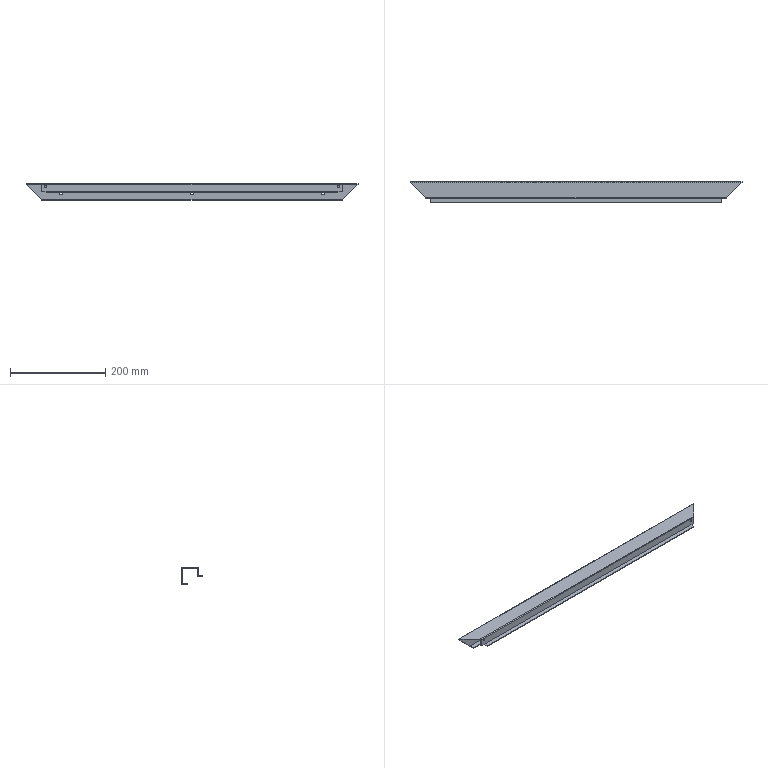Part | SolidWorks | features EdgeFlange 4, ICE 2, FlatPattern 1, LPattern 1, SMBaseFlange 1, SheetMetal 1 | 1 solid | 50 faces | box 697 x 43.5 x 35 mm | volume 100366 mm3 | plane 36 | cylinder 14 | commonest cylinder face diameters 10 x6 3 x4 4.5 x4
STEP:
#1=CARTESIAN_POINT('',(307.5,-16.,-3.25));
#2=VERTEX_POINT('',#1);
#3=CARTESIAN_POINT('',(307.5,-16.,-7.75));
#4=VERTEX_POINT('',#3);
#5=CARTESIAN_POINT('',(307.5,-16.,-5.5));
#6=DIRECTION('',(0.,-1.,0.));
#7=DIRECTION('',(0.,0.,-1.));
#8=AXIS2_PLACEMENT_3D('',#5,#6,#7);
#9=CIRCLE('',#8,2.25);
#10=EDGE_CURVE('',#2,#4,#9,.T.);
#11=ORIENTED_EDGE('',*,*,#10,.F.);
#12=CARTESIAN_POINT('',(307.5,-17.5,-3.25));
#13=VERTEX_POINT('',#12);
#14=CARTESIAN_POINT('',(307.5,-16.,-3.25));
#15=DIRECTION('',(0.,-1.,0.));
#16=VECTOR('',#15,1000.);
#17=LINE('',#14,#16);
#18=EDGE_CURVE('',#2,#13,#17,.T.);
#19=ORIENTED_EDGE('',*,*,#18,.T.);
#20=CARTESIAN_POINT('',(307.5,-17.5,-7.75));
#21=VERTEX_POINT('',#20);
#22=CARTESIAN_POINT('',(307.5,-17.5,-5.5));
#23=DIRECTION('',(0.,-1.,0.));
#24=DIRECTION('',(0.,0.,-1.));
#25=AXIS2_PLACEMENT_3D('',#22,#23,#24);
#26=CIRCLE('',#25,2.25);
#27=EDGE_CURVE('',#13,#21,#26,.T.);
#28=ORIENTED_EDGE('',*,*,#27,.T.);
#29=CARTESIAN_POINT('',(307.5,-16.,-7.75));
#30=DIRECTION('',(0.,-1.,0.));
#31=VECTOR('',#30,1000.);
#32=LINE('',#29,#31);
#33=EDGE_CURVE('',#4,#21,#32,.T.);
#34=ORIENTED_EDGE('',*,*,#33,.F.);
#35=EDGE_LOOP('',(#11,#19,#28,#34));
#36=FACE_OUTER_BOUND('',#35,.T.);
#37=CARTESIAN_POINT('',(307.5,-16.,-5.5));
#38=DIRECTION('',(0.,-1.,0.));
#39=DIRECTION('',(0.,0.,-1.));
#40=AXIS2_PLACEMENT_3D('',#37,#38,#39);
#41=CYLINDRICAL_SURFACE('',#40,2.25);
#42=ADVANCED_FACE('',(#36),#41,.F.);
#43=CARTESIAN_POINT('',(-307.5,-16.,-3.25));
#44=VERTEX_POINT('',#43);
#45=CARTESIAN_POINT('',(-307.5,-16.,-7.75));
#46=VERTEX_POINT('',#45);
#47=CARTESIAN_POINT('',(-307.5,-16.,-5.5));
#48=DIRECTION('',(0.,-1.,0.));
#49=DIRECTION('',(0.,0.,-1.));
#50=AXIS2_PLACEMENT_3D('',#47,#48,#49);
#51=CIRCLE('',#50,2.25);
#52=EDGE_CURVE('',#44,#46,#51,.T.);
#53=ORIENTED_EDGE('',*,*,#52,.F.);
#54=CARTESIAN_POINT('',(-307.5,-17.5,-3.25));
#55=VERTEX_POINT('',#54);
#56=CARTESIAN_POINT('',(-307.5,-16.,-3.25));
#57=DIRECTION('',(0.,-1.,0.));
#58=VECTOR('',#57,1000.);
#59=LINE('',#56,#58);
#60=EDGE_CURVE('',#44,#55,#59,.T.);
#61=ORIENTED_EDGE('',*,*,#60,.T.);
#62=CARTESIAN_POINT('',(-307.5,-17.5,-7.75));
#63=VERTEX_POINT('',#62);
#64=CARTESIAN_POINT('',(-307.5,-17.5,-5.5));
#65=DIRECTION('',(0.,-1.,0.));
#66=DIRECTION('',(0.,0.,-1.));
#67=AXIS2_PLACEMENT_3D('',#64,#65,#66);
#68=CIRCLE('',#67,2.25);
#69=EDGE_CURVE('',#55,#63,#68,.T.);
#70=ORIENTED_EDGE('',*,*,#69,.T.);
#71=CARTESIAN_POINT('',(-307.5,-16.,-7.75));
#72=DIRECTION('',(0.,-1.,0.));
#73=VECTOR('',#72,1000.);
#74=LINE('',#71,#73);
#75=EDGE_CURVE('',#46,#63,#74,.T.);
#76=ORIENTED_EDGE('',*,*,#75,.F.);
#77=EDGE_LOOP('',(#53,#61,#70,#76));
#78=FACE_OUTER_BOUND('',#77,.T.);
#79=CARTESIAN_POINT('',(-307.5,-16.,-5.5));
#80=DIRECTION('',(0.,-1.,0.));
#81=DIRECTION('',(0.,0.,-1.));
#82=AXIS2_PLACEMENT_3D('',#79,#80,#81);
#83=CYLINDRICAL_SURFACE('',#82,2.25);
#84=ADVANCED_FACE('',(#78),#83,.F.);
#85=CARTESIAN_POINT('',(275.,16.,-22.5));
#86=VERTEX_POINT('',#85);
#87=CARTESIAN_POINT('',(275.,16.,-12.5));
#88=VERTEX_POINT('',#87);
#89=CARTESIAN_POINT('',(275.,16.,-17.5));
#90=DIRECTION('',(0.,1.,0.));
#91=DIRECTION('',(0.,0.,1.));
#92=AXIS2_PLACEMENT_3D('',#89,#90,#91);
#93=CIRCLE('',#92,5.);
#94=EDGE_CURVE('',#86,#88,#93,.T.);
#95=ORIENTED_EDGE('',*,*,#94,.F.);
#96=CARTESIAN_POINT('',(275.,17.5,-22.5));
#97=VERTEX_POINT('',#96);
#98=CARTESIAN_POINT('',(275.,16.,-22.5));
#99=DIRECTION('',(0.,1.,0.));
#100=VECTOR('',#99,1000.);
#101=LINE('',#98,#100);
#102=EDGE_CURVE('',#86,#97,#101,.T.);
#103=ORIENTED_EDGE('',*,*,#102,.T.);
#104=CARTESIAN_POINT('',(275.,17.5,-12.5));
#105=VERTEX_POINT('',#104);
#106=CARTESIAN_POINT('',(275.,17.5,-17.5));
#107=DIRECTION('',(0.,1.,0.));
#108=DIRECTION('',(0.,0.,1.));
#109=AXIS2_PLACEMENT_3D('',#106,#107,#108);
#110=CIRCLE('',#109,5.);
#111=EDGE_CURVE('',#97,#105,#110,.T.);
#112=ORIENTED_EDGE('',*,*,#111,.T.);
#113=CARTESIAN_POINT('',(275.,16.,-12.5));
#114=DIRECTION('',(0.,1.,0.));
#115=VECTOR('',#114,1000.);
#116=LINE('',#113,#115);
#117=EDGE_CURVE('',#88,#105,#116,.T.);
#118=ORIENTED_EDGE('',*,*,#117,.F.);
#119=EDGE_LOOP('',(#95,#103,#112,#118));
#120=FACE_OUTER_BOUND('',#119,.T.);
#121=CARTESIAN_POINT('',(275.,16.,-17.5));
#122=DIRECTION('',(0.,1.,0.));
#123=DIRECTION('',(0.,0.,1.));
#124=AXIS2_PLACEMENT_3D('',#121,#122,#123);
#125=CYLINDRICAL_SURFACE('',#124,5.);
#126=ADVANCED_FACE('',(#120),#125,.F.);
#127=CARTESIAN_POINT('',(0.,16.,-22.5));
#128=VERTEX_POINT('',#127);
#129=CARTESIAN_POINT('',(0.,16.,-12.5));
#130=VERTEX_POINT('',#129);
#131=CARTESIAN_POINT('',(0.,16.,-17.5));
#132=DIRECTION('',(0.,1.,0.));
#133=DIRECTION('',(0.,0.,1.));
#134=AXIS2_PLACEMENT_3D('',#131,#132,#133);
#135=CIRCLE('',#134,5.);
#136=EDGE_CURVE('',#128,#130,#135,.T.);
#137=ORIENTED_EDGE('',*,*,#136,.F.);
#138=CARTESIAN_POINT('',(0.,17.5,-22.5));
#139=VERTEX_POINT('',#138);
#140=CARTESIAN_POINT('',(0.,16.,-22.5));
#141=DIRECTION('',(0.,1.,0.));
#142=VECTOR('',#141,1000.);
#143=LINE('',#140,#142);
#144=EDGE_CURVE('',#128,#139,#143,.T.);
#145=ORIENTED_EDGE('',*,*,#144,.T.);
#146=CARTESIAN_POINT('',(0.,17.5,-12.5));
#147=VERTEX_POINT('',#146);
#148=CARTESIAN_POINT('',(0.,17.5,-17.5));
#149=DIRECTION('',(0.,1.,0.));
#150=DIRECTION('',(0.,0.,1.));
#151=AXIS2_PLACEMENT_3D('',#148,#149,#150);
#152=CIRCLE('',#151,5.);
#153=EDGE_CURVE('',#139,#147,#152,.T.);
#154=ORIENTED_EDGE('',*,*,#153,.T.);
#155=CARTESIAN_POINT('',(0.,16.,-12.5));
#156=DIRECTION('',(0.,1.,0.));
#157=VECTOR('',#156,1000.);
#158=LINE('',#155,#157);
#159=EDGE_CURVE('',#130,#147,#158,.T.);
#160=ORIENTED_EDGE('',*,*,#159,.F.);
#161=EDGE_LOOP('',(#137,#145,#154,#160));
#162=FACE_OUTER_BOUND('',#161,.T.);
#163=CARTESIAN_POINT('',(0.,16.,-17.5));
#164=DIRECTION('',(0.,1.,0.));
#165=DIRECTION('',(0.,0.,1.));
#166=AXIS2_PLACEMENT_3D('',#163,#164,#165);
#167=CYLINDRICAL_SURFACE('',#166,5.);
#168=ADVANCED_FACE('',(#162),#167,.F.);
#169=CARTESIAN_POINT('',(-275.,16.,-22.5));
#170=VERTEX_POINT('',#169);
#171=CARTESIAN_POINT('',(-275.,16.,-12.5));
#172=VERTEX_POINT('',#171);
#173=CARTESIAN_POINT('',(-275.,16.,-17.5));
#174=DIRECTION('',(0.,1.,0.));
#175=DIRECTION('',(0.,0.,1.));
#176=AXIS2_PLACEMENT_3D('',#173,#174,#175);
#177=CIRCLE('',#176,5.);
#178=EDGE_CURVE('',#170,#172,#177,.T.);
#179=ORIENTED_EDGE('',*,*,#178,.F.);
#180=CARTESIAN_POINT('',(-275.,17.5,-22.5));
#181=VERTEX_POINT('',#180);
#182=CARTESIAN_POINT('',(-275.,16.,-22.5));
#183=DIRECTION('',(0.,1.,0.));
#184=VECTOR('',#183,1000.);
#185=LINE('',#182,#184);
#186=EDGE_CURVE('',#170,#181,#185,.T.);
#187=ORIENTED_EDGE('',*,*,#186,.T.);
#188=CARTESIAN_POINT('',(-275.,17.5,-12.5));
#189=VERTEX_POINT('',#188);
#190=CARTESIAN_POINT('',(-275.,17.5,-17.5));
#191=DIRECTION('',(0.,1.,0.));
#192=DIRECTION('',(0.,0.,1.));
#193=AXIS2_PLACEMENT_3D('',#190,#191,#192);
#194=CIRCLE('',#193,5.);
#195=EDGE_CURVE('',#181,#189,#194,.T.);
#196=ORIENTED_EDGE('',*,*,#195,.T.);
#197=CARTESIAN_POINT('',(-275.,16.,-12.5));
#198=DIRECTION('',(0.,1.,0.));
#199=VECTOR('',#198,1000.);
#200=LINE('',#197,#199);
#201=EDGE_CURVE('',#172,#189,#200,.T.);
#202=ORIENTED_EDGE('',*,*,#201,.F.);
#203=EDGE_LOOP('',(#179,#187,#196,#202));
#204=FACE_OUTER_BOUND('',#203,.T.);
#205=CARTESIAN_POINT('',(-275.,16.,-17.5));
#206=DIRECTION('',(0.,1.,0.));
#207=DIRECTION('',(0.,0.,1.));
#208=AXIS2_PLACEMENT_3D('',#205,#206,#207);
#209=CYLINDRICAL_SURFACE('',#208,5.);
#210=ADVANCED_FACE('',(#204),#209,.F.);
#211=CARTESIAN_POINT('',(-306.5,-16.,-17.));
#212=VERTEX_POINT('',#211);
#213=CARTESIAN_POINT('',(-315.,-16.,-17.));
#214=VERTEX_POINT('',#213);
#215=CARTESIAN_POINT('',(-315.,-16.,-17.));
#216=DIRECTION('',(-1.,0.,0.));
#217=VECTOR('',#216,1000.);
#218=LINE('',#215,#217);
#219=EDGE_CURVE('',#212,#214,#218,.T.);
#220=ORIENTED_EDGE('',*,*,#219,.F.);
#221=CARTESIAN_POINT('',(-306.5,-17.5,-17.));
#222=VERTEX_POINT('',#221);
#223=CARTESIAN_POINT('',(-306.5,-16.,-17.));
#224=DIRECTION('',(0.,-1.,0.));
#225=VECTOR('',#224,1000.);
#226=LINE('',#223,#225);
#227=EDGE_CURVE('',#212,#222,#226,.T.);
#228=ORIENTED_EDGE('',*,*,#227,.T.);
#229=CARTESIAN_POINT('',(-315.,-17.5,-17.));
#230=VERTEX_POINT('',#229);
#231=CARTESIAN_POINT('',(-315.,-17.5,-17.));
#232=DIRECTION('',(-1.,0.,0.));
#233=VECTOR('',#232,1000.);
#234=LINE('',#231,#233);
#235=EDGE_CURVE('',#222,#230,#234,.T.);
#236=ORIENTED_EDGE('',*,*,#235,.T.);
#237=CARTESIAN_POINT('',(-315.,-17.5,-17.));
#238=DIRECTION('',(0.,1.,0.));
#239=VECTOR('',#238,1000.);
#240=LINE('',#237,#239);
#241=EDGE_CURVE('',#230,#214,#240,.T.);
#242=ORIENTED_EDGE('',*,*,#241,.T.);
#243=EDGE_LOOP('',(#220,#228,#236,#242));
#244=FACE_OUTER_BOUND('',#243,.T.);
#245=CARTESIAN_POINT('',(-315.,-17.5,-17.));
#246=DIRECTION('',(0.,0.,-1.));
#247=DIRECTION('',(0.,1.,0.));
#248=AXIS2_PLACEMENT_3D('',#245,#246,#247);
#249=PLANE('',#248);
#250=ADVANCED_FACE('',(#244),#249,.T.);
#251=CARTESIAN_POINT('',(315.,-16.,0.));
#252=VERTEX_POINT('',#251);
#253=CARTESIAN_POINT('',(316.5,-16.,0.));
#254=VERTEX_POINT('',#253);
#255=CARTESIAN_POINT('',(316.5,-16.,0.));
#256=DIRECTION('',(1.,0.,0.));
#257=VECTOR('',#256,1000.);
#258=LINE('',#255,#257);
#259=EDGE_CURVE('',#252,#254,#258,.T.);
#260=ORIENTED_EDGE('',*,*,#259,.F.);
#261=CARTESIAN_POINT('',(315.,-16.,-1.5));
#262=VERTEX_POINT('',#261);
#263=CARTESIAN_POINT('',(315.,-16.,0.));
#264=DIRECTION('',(0.,0.,-1.));
#265=VECTOR('',#264,1000.);
#266=LINE('',#263,#265);
#267=EDGE_CURVE('',#252,#262,#266,.T.);
#268=ORIENTED_EDGE('',*,*,#267,.T.);
#269=CARTESIAN_POINT('',(316.5,-16.,-1.5));
#270=VERTEX_POINT('',#269);
#271=CARTESIAN_POINT('',(316.5,-16.,-1.5));
#272=DIRECTION('',(1.,0.,0.));
#273=VECTOR('',#272,1000.);
#274=LINE('',#271,#273);
#275=EDGE_CURVE('',#262,#270,#274,.T.);
#276=ORIENTED_EDGE('',*,*,#275,.T.);
#277=CARTESIAN_POINT('',(316.5,-16.,-1.5));
#278=DIRECTION('',(0.,0.,1.));
#279=VECTOR('',#278,1000.);
#280=LINE('',#277,#279);
#281=EDGE_CURVE('',#270,#254,#280,.T.);
#282=ORIENTED_EDGE('',*,*,#281,.T.);
#283=EDGE_LOOP('',(#260,#268,#276,#282));
#284=FACE_OUTER_BOUND('',#283,.T.);
#285=CARTESIAN_POINT('',(316.5,-16.,-1.5));
#286=DIRECTION('',(0.,-1.,0.));
#287=DIRECTION('',(1.,0.,0.));
#288=AXIS2_PLACEMENT_3D('',#285,#286,#287);
#289=PLANE('',#288);
#290=ADVANCED_FACE('',(#284),#289,.T.);
#291=CARTESIAN_POINT('',(-316.5,17.5,-33.5));
#292=VERTEX_POINT('',#291);
#293=CARTESIAN_POINT('',(-315.,17.5,-33.5));
#294=VERTEX_POINT('',#293);
#295=CARTESIAN_POINT('',(316.5,17.5,-33.5));
#296=DIRECTION('',(1.,0.,0.));
#297=VECTOR('',#296,1000.);
#298=LINE('',#295,#297);
#299=EDGE_CURVE('',#292,#294,#298,.T.);
#300=ORIENTED_EDGE('',*,*,#299,.T.);
#301=CARTESIAN_POINT('',(-315.,16.,-33.5));
#302=VERTEX_POINT('',#301);
#303=CARTESIAN_POINT('',(-315.,17.5,-33.5));
#304=DIRECTION('',(0.,-1.,0.));
#305=VECTOR('',#304,1000.);
#306=LINE('',#303,#305);
#307=EDGE_CURVE('',#294,#302,#306,.T.);
#308=ORIENTED_EDGE('',*,*,#307,.T.);
#309=CARTESIAN_POINT('',(-316.5,16.,-33.5));
#310=VERTEX_POINT('',#309);
#311=CARTESIAN_POINT('',(316.5,16.,-33.5));
#312=DIRECTION('',(1.,0.,0.));
#313=VECTOR('',#312,1000.);
#314=LINE('',#311,#313);
#315=EDGE_CURVE('',#310,#302,#314,.T.);
#316=ORIENTED_EDGE('',*,*,#315,.F.);
#317=CARTESIAN_POINT('',(-316.5,17.5,-33.5));
#318=DIRECTION('',(0.,-1.,0.));
#319=VECTOR('',#318,1000.);
#320=LINE('',#317,#319);
#321=EDGE_CURVE('',#292,#310,#320,.T.);
#322=ORIENTED_EDGE('',*,*,#321,.F.);
#323=EDGE_LOOP('',(#300,#308,#316,#322));
#324=FACE_OUTER_BOUND('',#323,.T.);
#325=CARTESIAN_POINT('',(316.5,17.5,-33.5));
#326=DIRECTION('',(0.,0.,-1.));
#327=DIRECTION('',(0.,1.,0.));
#328=AXIS2_PLACEMENT_3D('',#325,#326,#327);
#329=PLANE('',#328);
#330=ADVANCED_FACE('',(#324),#329,.T.);
#331=CARTESIAN_POINT('',(-348.5,16.,0.));
#332=VERTEX_POINT('',#331);
#333=CARTESIAN_POINT('',(-316.5,-16.,0.));
#334=VERTEX_POINT('',#333);
#335=CARTESIAN_POINT('',(-316.5,-16.,0.));
#336=DIRECTION('',(0.7071,-0.7071,0.));
#337=VECTOR('',#336,1000.);
#338=LINE('',#335,#337);
#339=EDGE_CURVE('',#332,#334,#338,.T.);
#340=ORIENTED_EDGE('',*,*,#339,.F.);
#341=CARTESIAN_POINT('',(-348.5,16.,-1.5));
#342=VERTEX_POINT('',#341);
#343=CARTESIAN_POINT('',(-348.5,16.,-1.5));
#344=DIRECTION('',(0.,0.,1.));
#345=VECTOR('',#344,1000.);
#346=LINE('',#343,#345);
#347=EDGE_CURVE('',#342,#332,#346,.T.);
#348=ORIENTED_EDGE('',*,*,#347,.F.);
#349=CARTESIAN_POINT('',(-316.5,-16.,-1.5));
#350=VERTEX_POINT('',#349);
#351=CARTESIAN_POINT('',(-316.5,-16.,-1.5));
#352=DIRECTION('',(0.7071,-0.7071,0.));
#353=VECTOR('',#352,1000.);
#354=LINE('',#351,#353);
#355=EDGE_CURVE('',#342,#350,#354,.T.);
#356=ORIENTED_EDGE('',*,*,#355,.T.);
#357=CARTESIAN_POINT('',(-316.5,-16.,-1.5));
#358=DIRECTION('',(0.,0.,1.));
#359=VECTOR('',#358,1000.);
#360=LINE('',#357,#359);
#361=EDGE_CURVE('',#350,#334,#360,.T.);
#362=ORIENTED_EDGE('',*,*,#361,.T.);
#363=EDGE_LOOP('',(#340,#348,#356,#362));
#364=FACE_OUTER_BOUND('',#363,.T.);
#365=CARTESIAN_POINT('',(-316.5,-16.,-1.5));
#366=DIRECTION('',(-0.7071,-0.7071,0.));
#367=DIRECTION('',(0.7071,-0.7071,0.));
#368=AXIS2_PLACEMENT_3D('',#365,#366,#367);
#369=PLANE('',#368);
#370=ADVANCED_FACE('',(#364),#369,.T.);
#371=CARTESIAN_POINT('',(348.5,16.,0.));
#372=VERTEX_POINT('',#371);
#373=CARTESIAN_POINT('',(348.5,16.,0.));
#374=DIRECTION('',(0.7071,0.7071,0.));
#375=VECTOR('',#374,1000.);
#376=LINE('',#373,#375);
#377=EDGE_CURVE('',#254,#372,#376,.T.);
#378=ORIENTED_EDGE('',*,*,#377,.F.);
#379=ORIENTED_EDGE('',*,*,#281,.F.);
#380=CARTESIAN_POINT('',(348.5,16.,-1.5));
#381=VERTEX_POINT('',#380);
#382=CARTESIAN_POINT('',(348.5,16.,-1.5));
#383=DIRECTION('',(0.7071,0.7071,0.));
#384=VECTOR('',#383,1000.);
#385=LINE('',#382,#384);
#386=EDGE_CURVE('',#270,#381,#385,.T.);
#387=ORIENTED_EDGE('',*,*,#386,.T.);
#388=CARTESIAN_POINT('',(348.5,16.,-1.5));
#389=DIRECTION('',(0.,0.,1.));
#390=VECTOR('',#389,1000.);
#391=LINE('',#388,#390);
#392=EDGE_CURVE('',#381,#372,#391,.T.);
#393=ORIENTED_EDGE('',*,*,#392,.T.);
#394=EDGE_LOOP('',(#378,#379,#387,#393));
#395=FACE_OUTER_BOUND('',#394,.T.);
#396=CARTESIAN_POINT('',(348.5,16.,-1.5));
#397=DIRECTION('',(0.7071,-0.7071,0.));
#398=DIRECTION('',(0.7071,0.7071,0.));
#399=AXIS2_PLACEMENT_3D('',#396,#397,#398);
#400=PLANE('',#399);
#401=ADVANCED_FACE('',(#395),#400,.T.);
#402=CARTESIAN_POINT('',(-315.,-16.,0.));
#403=VERTEX_POINT('',#402);
#404=CARTESIAN_POINT('',(-315.,-16.,-1.5));
#405=VERTEX_POINT('',#404);
#406=CARTESIAN_POINT('',(-315.,-16.,0.));
#407=DIRECTION('',(0.,0.,-1.));
#408=VECTOR('',#407,1000.);
#409=LINE('',#406,#408);
#410=EDGE_CURVE('',#403,#405,#409,.T.);
#411=ORIENTED_EDGE('',*,*,#410,.F.);
#412=CARTESIAN_POINT('',(316.5,-16.,0.));
#413=DIRECTION('',(1.,0.,0.));
#414=VECTOR('',#413,1000.);
#415=LINE('',#412,#414);
#416=EDGE_CURVE('',#334,#403,#415,.T.);
#417=ORIENTED_EDGE('',*,*,#416,.F.);
#418=ORIENTED_EDGE('',*,*,#361,.F.);
#419=CARTESIAN_POINT('',(316.5,-16.,-1.5));
#420=DIRECTION('',(1.,0.,0.));
#421=VECTOR('',#420,1000.);
#422=LINE('',#419,#421);
#423=EDGE_CURVE('',#350,#405,#422,.T.);
#424=ORIENTED_EDGE('',*,*,#423,.T.);
#425=EDGE_LOOP('',(#411,#417,#418,#424));
#426=FACE_OUTER_BOUND('',#425,.T.);
#427=CARTESIAN_POINT('',(316.5,-16.,-1.5));
#428=DIRECTION('',(0.,-1.,0.));
#429=DIRECTION('',(1.,0.,0.));
#430=AXIS2_PLACEMENT_3D('',#427,#428,#429);
#431=PLANE('',#430);
#432=ADVANCED_FACE('',(#426),#431,.T.);
#433=ORIENTED_EDGE('',*,*,#355,.F.);
#434=CARTESIAN_POINT('',(-348.5,16.,-1.5));
#435=DIRECTION('',(-1.,0.,0.));
#436=VECTOR('',#435,1000.);
#437=LINE('',#434,#436);
#438=EDGE_CURVE('',#381,#342,#437,.T.);
#439=ORIENTED_EDGE('',*,*,#438,.F.);
#440=ORIENTED_EDGE('',*,*,#386,.F.);
#441=ORIENTED_EDGE('',*,*,#275,.F.);
#442=CARTESIAN_POINT('',(315.,-16.,-1.5));
#443=DIRECTION('',(1.,0.,0.));
#444=VECTOR('',#443,1000.);
#445=LINE('',#442,#444);
#446=EDGE_CURVE('',#405,#262,#445,.T.);
#447=ORIENTED_EDGE('',*,*,#446,.F.);
#448=ORIENTED_EDGE('',*,*,#423,.F.);
#449=EDGE_LOOP('',(#433,#439,#440,#441,#447,#448));
#450=FACE_OUTER_BOUND('',#449,.T.);
#451=CARTESIAN_POINT('',(0.,-332.5,-1.5));
#452=DIRECTION('',(0.,0.,1.));
#453=DIRECTION('',(1.,0.,0.));
#454=AXIS2_PLACEMENT_3D('',#451,#452,#453);
#455=PLANE('',#454);
#456=ADVANCED_FACE('',(#450),#455,.F.);
#457=ORIENTED_EDGE('',*,*,#339,.T.);
#458=ORIENTED_EDGE('',*,*,#416,.T.);
#459=CARTESIAN_POINT('',(315.,-16.,0.));
#460=DIRECTION('',(1.,0.,0.));
#461=VECTOR('',#460,1000.);
#462=LINE('',#459,#461);
#463=EDGE_CURVE('',#403,#252,#462,.T.);
#464=ORIENTED_EDGE('',*,*,#463,.T.);
#465=ORIENTED_EDGE('',*,*,#259,.T.);
#466=ORIENTED_EDGE('',*,*,#377,.T.);
#467=CARTESIAN_POINT('',(-348.5,16.,0.));
#468=DIRECTION('',(-1.,0.,0.));
#469=VECTOR('',#468,1000.);
#470=LINE('',#467,#469);
#471=EDGE_CURVE('',#372,#332,#470,.T.);
#472=ORIENTED_EDGE('',*,*,#471,.T.);
#473=EDGE_LOOP('',(#457,#458,#464,#465,#466,#472));
#474=FACE_OUTER_BOUND('',#473,.T.);
#475=CARTESIAN_POINT('',(0.,-332.5,0.));
#476=DIRECTION('',(0.,0.,1.));
#477=DIRECTION('',(1.,0.,0.));
#478=AXIS2_PLACEMENT_3D('',#475,#476,#477);
#479=PLANE('',#478);
#480=ADVANCED_FACE('',(#474),#479,.T.);
#481=CARTESIAN_POINT('',(348.5,17.5,-1.5));
#482=VERTEX_POINT('',#481);
#483=CARTESIAN_POINT('',(348.5,16.,-1.5));
#484=DIRECTION('',(-1.,0.,0.));
#485=DIRECTION('',(0.,0.,1.));
#486=AXIS2_PLACEMENT_3D('',#483,#484,#485);
#487=CIRCLE('',#486,1.5);
#488=EDGE_CURVE('',#372,#482,#487,.T.);
#489=ORIENTED_EDGE('',*,*,#488,.F.);
#490=ORIENTED_EDGE('',*,*,#392,.F.);
#491=CARTESIAN_POINT('',(348.5,17.5,-1.5));
#492=DIRECTION('',(0.,-1.,0.));
#493=VECTOR('',#492,1000.);
#494=LINE('',#491,#493);
#495=EDGE_CURVE('',#482,#381,#494,.T.);
#496=ORIENTED_EDGE('',*,*,#495,.F.);
#497=EDGE_LOOP('',(#489,#490,#496));
#498=FACE_OUTER_BOUND('',#497,.T.);
#499=CARTESIAN_POINT('',(348.5,16.,0.));
#500=DIRECTION('',(1.,0.,0.));
#501=DIRECTION('',(0.,0.,-1.));
#502=AXIS2_PLACEMENT_3D('',#499,#500,#501);
#503=PLANE('',#502);
#504=ADVANCED_FACE('',(#498),#503,.T.);
#505=CARTESIAN_POINT('',(-348.5,17.5,-1.5));
#506=VERTEX_POINT('',#505);
#507=CARTESIAN_POINT('',(-348.5,16.,-1.5));
#508=DIRECTION('',(-1.,0.,0.));
#509=DIRECTION('',(0.,0.,1.));
#510=AXIS2_PLACEMENT_3D('',#507,#508,#509);
#511=CIRCLE('',#510,1.5);
#512=EDGE_CURVE('',#332,#506,#511,.T.);
#513=ORIENTED_EDGE('',*,*,#512,.F.);
#514=ORIENTED_EDGE('',*,*,#471,.F.);
#515=ORIENTED_EDGE('',*,*,#488,.T.);
#516=CARTESIAN_POINT('',(-348.5,17.5,-1.5));
#517=DIRECTION('',(-1.,0.,0.));
#518=VECTOR('',#517,1000.);
#519=LINE('',#516,#518);
#520=EDGE_CURVE('',#482,#506,#519,.T.);
#521=ORIENTED_EDGE('',*,*,#520,.T.);
#522=EDGE_LOOP('',(#513,#514,#515,#521));
#523=FACE_OUTER_BOUND('',#522,.T.);
#524=CARTESIAN_POINT('',(-348.5,16.,-1.5));
#525=DIRECTION('',(-1.,0.,0.));
#526=DIRECTION('',(0.,0.,1.));
#527=AXIS2_PLACEMENT_3D('',#524,#525,#526);
#528=CYLINDRICAL_SURFACE('',#527,1.5);
#529=ADVANCED_FACE('',(#523),#528,.T.);
#530=ORIENTED_EDGE('',*,*,#347,.T.);
#531=ORIENTED_EDGE('',*,*,#512,.T.);
#532=CARTESIAN_POINT('',(-348.5,17.5,-1.5));
#533=DIRECTION('',(0.,-1.,0.));
#534=VECTOR('',#533,1000.);
#535=LINE('',#532,#534);
#536=EDGE_CURVE('',#506,#342,#535,.T.);
#537=ORIENTED_EDGE('',*,*,#536,.T.);
#538=EDGE_LOOP('',(#530,#531,#537));
#539=FACE_OUTER_BOUND('',#538,.T.);
#540=CARTESIAN_POINT('',(-348.5,16.,0.));
#541=DIRECTION('',(1.,0.,0.));
#542=DIRECTION('',(0.,0.,-1.));
#543=AXIS2_PLACEMENT_3D('',#540,#541,#542);
#544=PLANE('',#543);
#545=ADVANCED_FACE('',(#539),#544,.F.);
#546=CARTESIAN_POINT('',(316.5,16.,-33.5));
#547=VERTEX_POINT('',#546);
#548=CARTESIAN_POINT('',(348.5,16.,-1.5));
#549=DIRECTION('',(0.7071,0.,0.7071));
#550=VECTOR('',#549,1000.);
#551=LINE('',#548,#550);
#552=EDGE_CURVE('',#547,#381,#551,.T.);
#553=ORIENTED_EDGE('',*,*,#552,.F.);
#554=CARTESIAN_POINT('',(316.5,17.5,-33.5));
#555=VERTEX_POINT('',#554);
#556=CARTESIAN_POINT('',(316.5,17.5,-33.5));
#557=DIRECTION('',(0.,-1.,0.));
#558=VECTOR('',#557,1000.);
#559=LINE('',#556,#558);
#560=EDGE_CURVE('',#555,#547,#559,.T.);
#561=ORIENTED_EDGE('',*,*,#560,.F.);
#562=CARTESIAN_POINT('',(348.5,17.5,-1.5));
#563=DIRECTION('',(0.7071,0.,0.7071));
#564=VECTOR('',#563,1000.);
#565=LINE('',#562,#564);
#566=EDGE_CURVE('',#555,#482,#565,.T.);
#567=ORIENTED_EDGE('',*,*,#566,.T.);
#568=ORIENTED_EDGE('',*,*,#495,.T.);
#569=EDGE_LOOP('',(#553,#561,#567,#568));
#570=FACE_OUTER_BOUND('',#569,.T.);
#571=CARTESIAN_POINT('',(348.5,17.5,-1.5));
#572=DIRECTION('',(0.7071,0.,-0.7071));
#573=DIRECTION('',(-0.7071,0.,-0.7071));
#574=AXIS2_PLACEMENT_3D('',#571,#572,#573);
#575=PLANE('',#574);
#576=ADVANCED_FACE('',(#570),#575,.T.);
#577=CARTESIAN_POINT('',(315.,17.5,-33.5));
#578=VERTEX_POINT('',#577);
#579=CARTESIAN_POINT('',(315.,16.,-33.5));
#580=VERTEX_POINT('',#579);
#581=CARTESIAN_POINT('',(315.,17.5,-33.5));
#582=DIRECTION('',(0.,-1.,0.));
#583=VECTOR('',#582,1000.);
#584=LINE('',#581,#583);
#585=EDGE_CURVE('',#578,#580,#584,.T.);
#586=ORIENTED_EDGE('',*,*,#585,.F.);
#587=CARTESIAN_POINT('',(316.5,17.5,-33.5));
#588=DIRECTION('',(1.,0.,0.));
#589=VECTOR('',#588,1000.);
#590=LINE('',#587,#589);
#591=EDGE_CURVE('',#578,#555,#590,.T.);
#592=ORIENTED_EDGE('',*,*,#591,.T.);
#593=ORIENTED_EDGE('',*,*,#560,.T.);
#594=CARTESIAN_POINT('',(316.5,16.,-33.5));
#595=DIRECTION('',(1.,0.,0.));
#596=VECTOR('',#595,1000.);
#597=LINE('',#594,#596);
#598=EDGE_CURVE('',#580,#547,#597,.T.);
#599=ORIENTED_EDGE('',*,*,#598,.F.);
#600=EDGE_LOOP('',(#586,#592,#593,#599));
#601=FACE_OUTER_BOUND('',#600,.T.);
#602=CARTESIAN_POINT('',(316.5,17.5,-33.5));
#603=DIRECTION('',(0.,0.,-1.));
#604=DIRECTION('',(0.,1.,0.));
#605=AXIS2_PLACEMENT_3D('',#602,#603,#604);
#606=PLANE('',#605);
#607=ADVANCED_FACE('',(#601),#606,.T.);
#608=CARTESIAN_POINT('',(-316.5,16.,-33.5));
#609=DIRECTION('',(0.7071,0.,-0.7071));
#610=VECTOR('',#609,1000.);
#611=LINE('',#608,#610);
#612=EDGE_CURVE('',#342,#310,#611,.T.);
#613=ORIENTED_EDGE('',*,*,#612,.F.);
#614=ORIENTED_EDGE('',*,*,#536,.F.);
#615=CARTESIAN_POINT('',(-316.5,17.5,-33.5));
#616=DIRECTION('',(0.7071,0.,-0.7071));
#617=VECTOR('',#616,1000.);
#618=LINE('',#615,#617);
#619=EDGE_CURVE('',#506,#292,#618,.T.);
#620=ORIENTED_EDGE('',*,*,#619,.T.);
#621=ORIENTED_EDGE('',*,*,#321,.T.);
#622=EDGE_LOOP('',(#613,#614,#620,#621));
#623=FACE_OUTER_BOUND('',#622,.T.);
#624=CARTESIAN_POINT('',(-316.5,17.5,-33.5));
#625=DIRECTION('',(-0.7071,0.,-0.7071));
#626=DIRECTION('',(-0.7071,0.,0.7071));
#627=AXIS2_PLACEMENT_3D('',#624,#625,#626);
#628=PLANE('',#627);
#629=ADVANCED_FACE('',(#623),#628,.T.);
#630=CARTESIAN_POINT('',(275.,17.5,-17.5));
#631=DIRECTION('',(0.,1.,0.));
#632=DIRECTION('',(0.,0.,1.));
#633=AXIS2_PLACEMENT_3D('',#630,#631,#632);
#634=CIRCLE('',#633,5.);
#635=EDGE_CURVE('',#105,#97,#634,.T.);
#636=ORIENTED_EDGE('',*,*,#635,.F.);
#637=ORIENTED_EDGE('',*,*,#111,.F.);
#638=EDGE_LOOP('',(#636,#637));
#639=FACE_BOUND('',#638,.T.);
#640=CARTESIAN_POINT('',(0.,17.5,-17.5));
#641=DIRECTION('',(0.,1.,0.));
#642=DIRECTION('',(0.,0.,1.));
#643=AXIS2_PLACEMENT_3D('',#640,#641,#642);
#644=CIRCLE('',#643,5.);
#645=EDGE_CURVE('',#147,#139,#644,.T.);
#646=ORIENTED_EDGE('',*,*,#645,.F.);
#647=ORIENTED_EDGE('',*,*,#153,.F.);
#648=EDGE_LOOP('',(#646,#647));
#649=FACE_BOUND('',#648,.T.);
#650=CARTESIAN_POINT('',(-275.,17.5,-17.5));
#651=DIRECTION('',(0.,1.,0.));
#652=DIRECTION('',(0.,0.,1.));
#653=AXIS2_PLACEMENT_3D('',#650,#651,#652);
#654=CIRCLE('',#653,5.);
#655=EDGE_CURVE('',#189,#181,#654,.T.);
#656=ORIENTED_EDGE('',*,*,#655,.F.);
#657=ORIENTED_EDGE('',*,*,#195,.F.);
#658=EDGE_LOOP('',(#656,#657));
#659=FACE_BOUND('',#658,.T.);
#660=ORIENTED_EDGE('',*,*,#520,.F.);
#661=ORIENTED_EDGE('',*,*,#566,.F.);
#662=ORIENTED_EDGE('',*,*,#591,.F.);
#663=CARTESIAN_POINT('',(-315.,17.5,-33.5));
#664=DIRECTION('',(-1.,0.,0.));
#665=VECTOR('',#664,1000.);
#666=LINE('',#663,#665);
#667=EDGE_CURVE('',#578,#294,#666,.T.);
#668=ORIENTED_EDGE('',*,*,#667,.T.);
#669=ORIENTED_EDGE('',*,*,#299,.F.);
#670=ORIENTED_EDGE('',*,*,#619,.F.);
#671=EDGE_LOOP('',(#660,#661,#662,#668,#669,#670));
#672=FACE_OUTER_BOUND('',#671,.T.);
#673=CARTESIAN_POINT('',(348.5,17.5,-1.5));
#674=DIRECTION('',(0.,1.,0.));
#675=DIRECTION('',(0.,0.,1.));
#676=AXIS2_PLACEMENT_3D('',#673,#674,#675);
#677=PLANE('',#676);
#678=ADVANCED_FACE('',(#639,#649,#659,#672),#677,.T.);
#679=CARTESIAN_POINT('',(275.,16.,-17.5));
#680=DIRECTION('',(0.,1.,0.));
#681=DIRECTION('',(0.,0.,1.));
#682=AXIS2_PLACEMENT_3D('',#679,#680,#681);
#683=CIRCLE('',#682,5.);
#684=EDGE_CURVE('',#88,#86,#683,.T.);
#685=ORIENTED_EDGE('',*,*,#684,.T.);
#686=ORIENTED_EDGE('',*,*,#94,.T.);
#687=EDGE_LOOP('',(#685,#686));
#688=FACE_BOUND('',#687,.T.);
#689=CARTESIAN_POINT('',(0.,16.,-17.5));
#690=DIRECTION('',(0.,1.,0.));
#691=DIRECTION('',(0.,0.,1.));
#692=AXIS2_PLACEMENT_3D('',#689,#690,#691);
#693=CIRCLE('',#692,5.);
#694=EDGE_CURVE('',#130,#128,#693,.T.);
#695=ORIENTED_EDGE('',*,*,#694,.T.);
#696=ORIENTED_EDGE('',*,*,#136,.T.);
#697=EDGE_LOOP('',(#695,#696));
#698=FACE_BOUND('',#697,.T.);
#699=CARTESIAN_POINT('',(-275.,16.,-17.5));
#700=DIRECTION('',(0.,1.,0.));
#701=DIRECTION('',(0.,0.,1.));
#702=AXIS2_PLACEMENT_3D('',#699,#700,#701);
#703=CIRCLE('',#702,5.);
#704=EDGE_CURVE('',#172,#170,#703,.T.);
#705=ORIENTED_EDGE('',*,*,#704,.T.);
#706=ORIENTED_EDGE('',*,*,#178,.T.);
#707=EDGE_LOOP('',(#705,#706));
#708=FACE_BOUND('',#707,.T.);
#709=ORIENTED_EDGE('',*,*,#438,.T.);
#710=ORIENTED_EDGE('',*,*,#612,.T.);
#711=ORIENTED_EDGE('',*,*,#315,.T.);
#712=CARTESIAN_POINT('',(-315.,16.,-33.5));
#713=DIRECTION('',(-1.,0.,0.));
#714=VECTOR('',#713,1000.);
#715=LINE('',#712,#714);
#716=EDGE_CURVE('',#580,#302,#715,.T.);
#717=ORIENTED_EDGE('',*,*,#716,.F.);
#718=ORIENTED_EDGE('',*,*,#598,.T.);
#719=ORIENTED_EDGE('',*,*,#552,.T.);
#720=EDGE_LOOP('',(#709,#710,#711,#717,#718,#719));
#721=FACE_OUTER_BOUND('',#720,.T.);
#722=CARTESIAN_POINT('',(348.5,16.,-1.5));
#723=DIRECTION('',(0.,1.,0.));
#724=DIRECTION('',(0.,0.,1.));
#725=AXIS2_PLACEMENT_3D('',#722,#723,#724);
#726=PLANE('',#725);
#727=ADVANCED_FACE('',(#688,#698,#708,#721),#726,.F.);
#728=CARTESIAN_POINT('',(315.,16.,-35.));
#729=VERTEX_POINT('',#728);
#730=CARTESIAN_POINT('',(315.,16.,-33.5));
#731=DIRECTION('',(-1.,0.,0.));
#732=DIRECTION('',(0.,-1.,0.));
#733=AXIS2_PLACEMENT_3D('',#730,#731,#732);
#734=CIRCLE('',#733,1.5);
#735=EDGE_CURVE('',#578,#729,#734,.T.);
#736=ORIENTED_EDGE('',*,*,#735,.F.);
#737=ORIENTED_EDGE('',*,*,#585,.T.);
#738=CARTESIAN_POINT('',(315.,16.,-35.));
#739=DIRECTION('',(0.,0.,1.));
#740=VECTOR('',#739,1000.);
#741=LINE('',#738,#740);
#742=EDGE_CURVE('',#729,#580,#741,.T.);
#743=ORIENTED_EDGE('',*,*,#742,.F.);
#744=EDGE_LOOP('',(#736,#737,#743));
#745=FACE_OUTER_BOUND('',#744,.T.);
#746=CARTESIAN_POINT('',(315.,17.5,-33.5));
#747=DIRECTION('',(1.,0.,0.));
#748=DIRECTION('',(0.,1.,0.));
#749=AXIS2_PLACEMENT_3D('',#746,#747,#748);
#750=PLANE('',#749);
#751=ADVANCED_FACE('',(#745),#750,.T.);
#752=CARTESIAN_POINT('',(-315.,16.,-35.));
#753=VERTEX_POINT('',#752);
#754=CARTESIAN_POINT('',(-315.,16.,-33.5));
#755=DIRECTION('',(-1.,0.,0.));
#756=DIRECTION('',(0.,-1.,0.));
#757=AXIS2_PLACEMENT_3D('',#754,#755,#756);
#758=CIRCLE('',#757,1.5);
#759=EDGE_CURVE('',#294,#753,#758,.T.);
#760=ORIENTED_EDGE('',*,*,#759,.F.);
#761=ORIENTED_EDGE('',*,*,#667,.F.);
#762=ORIENTED_EDGE('',*,*,#735,.T.);
#763=CARTESIAN_POINT('',(-315.,16.,-35.));
#764=DIRECTION('',(-1.,0.,0.));
#765=VECTOR('',#764,1000.);
#766=LINE('',#763,#765);
#767=EDGE_CURVE('',#729,#753,#766,.T.);
#768=ORIENTED_EDGE('',*,*,#767,.T.);
#769=EDGE_LOOP('',(#760,#761,#762,#768));
#770=FACE_OUTER_BOUND('',#769,.T.);
#771=CARTESIAN_POINT('',(-315.,16.,-33.5));
#772=DIRECTION('',(-1.,0.,0.));
#773=DIRECTION('',(0.,-1.,0.));
#774=AXIS2_PLACEMENT_3D('',#771,#772,#773);
#775=CYLINDRICAL_SURFACE('',#774,1.5);
#776=ADVANCED_FACE('',(#770),#775,.T.);
#777=ORIENTED_EDGE('',*,*,#307,.F.);
#778=ORIENTED_EDGE('',*,*,#759,.T.);
#779=CARTESIAN_POINT('',(-315.,16.,-35.));
#780=DIRECTION('',(0.,0.,1.));
#781=VECTOR('',#780,1000.);
#782=LINE('',#779,#781);
#783=EDGE_CURVE('',#753,#302,#782,.T.);
#784=ORIENTED_EDGE('',*,*,#783,.T.);
#785=EDGE_LOOP('',(#777,#778,#784));
#786=FACE_OUTER_BOUND('',#785,.T.);
#787=CARTESIAN_POINT('',(-315.,17.5,-33.5));
#788=DIRECTION('',(1.,0.,0.));
#789=DIRECTION('',(0.,1.,0.));
#790=AXIS2_PLACEMENT_3D('',#787,#788,#789);
#791=PLANE('',#790);
#792=ADVANCED_FACE('',(#786),#791,.F.);
#793=CARTESIAN_POINT('',(315.,5.5,-33.5));
#794=VERTEX_POINT('',#793);
#795=CARTESIAN_POINT('',(315.,16.,-33.5));
#796=DIRECTION('',(0.,1.,0.));
#797=VECTOR('',#796,1000.);
#798=LINE('',#795,#797);
#799=EDGE_CURVE('',#794,#580,#798,.T.);
#800=ORIENTED_EDGE('',*,*,#799,.F.);
#801=CARTESIAN_POINT('',(315.,5.5,-35.));
#802=VERTEX_POINT('',#801);
#803=CARTESIAN_POINT('',(315.,5.5,-35.));
#804=DIRECTION('',(0.,0.,1.));
#805=VECTOR('',#804,1000.);
#806=LINE('',#803,#805);
#807=EDGE_CURVE('',#802,#794,#806,.T.);
#808=ORIENTED_EDGE('',*,*,#807,.F.);
#809=CARTESIAN_POINT('',(315.,16.,-35.));
#810=DIRECTION('',(0.,1.,0.));
#811=VECTOR('',#810,1000.);
#812=LINE('',#809,#811);
#813=EDGE_CURVE('',#802,#729,#812,.T.);
#814=ORIENTED_EDGE('',*,*,#813,.T.);
#815=ORIENTED_EDGE('',*,*,#742,.T.);
#816=EDGE_LOOP('',(#800,#808,#814,#815));
#817=FACE_OUTER_BOUND('',#816,.T.);
#818=CARTESIAN_POINT('',(315.,16.,-35.));
#819=DIRECTION('',(1.,0.,0.));
#820=DIRECTION('',(0.,0.,-1.));
#821=AXIS2_PLACEMENT_3D('',#818,#819,#820);
#822=PLANE('',#821);
#823=ADVANCED_FACE('',(#817),#822,.T.);
#824=CARTESIAN_POINT('',(-315.,5.5,-33.5));
#825=VERTEX_POINT('',#824);
#826=CARTESIAN_POINT('',(315.,5.5,-33.5));
#827=DIRECTION('',(1.,0.,0.));
#828=VECTOR('',#827,1000.);
#829=LINE('',#826,#828);
#830=EDGE_CURVE('',#825,#794,#829,.T.);
#831=ORIENTED_EDGE('',*,*,#830,.F.);
#832=CARTESIAN_POINT('',(-315.,5.5,-35.));
#833=VERTEX_POINT('',#832);
#834=CARTESIAN_POINT('',(-315.,5.5,-35.));
#835=DIRECTION('',(0.,0.,1.));
#836=VECTOR('',#835,1000.);
#837=LINE('',#834,#836);
#838=EDGE_CURVE('',#833,#825,#837,.T.);
#839=ORIENTED_EDGE('',*,*,#838,.F.);
#840=CARTESIAN_POINT('',(315.,5.5,-35.));
#841=DIRECTION('',(1.,0.,0.));
#842=VECTOR('',#841,1000.);
#843=LINE('',#840,#842);
#844=EDGE_CURVE('',#833,#802,#843,.T.);
#845=ORIENTED_EDGE('',*,*,#844,.T.);
#846=ORIENTED_EDGE('',*,*,#807,.T.);
#847=EDGE_LOOP('',(#831,#839,#845,#846));
#848=FACE_OUTER_BOUND('',#847,.T.);
#849=CARTESIAN_POINT('',(315.,5.5,-35.));
#850=DIRECTION('',(0.,-1.,0.));
#851=DIRECTION('',(0.,0.,-1.));
#852=AXIS2_PLACEMENT_3D('',#849,#850,#851);
#853=PLANE('',#852);
#854=ADVANCED_FACE('',(#848),#853,.T.);
#855=CARTESIAN_POINT('',(-315.,5.5,-33.5));
#856=DIRECTION('',(0.,-1.,0.));
#857=VECTOR('',#856,1000.);
#858=LINE('',#855,#857);
#859=EDGE_CURVE('',#302,#825,#858,.T.);
#860=ORIENTED_EDGE('',*,*,#859,.F.);
#861=ORIENTED_EDGE('',*,*,#783,.F.);
#862=CARTESIAN_POINT('',(-315.,5.5,-35.));
#863=DIRECTION('',(0.,-1.,0.));
#864=VECTOR('',#863,1000.);
#865=LINE('',#862,#864);
#866=EDGE_CURVE('',#753,#833,#865,.T.);
#867=ORIENTED_EDGE('',*,*,#866,.T.);
#868=ORIENTED_EDGE('',*,*,#838,.T.);
#869=EDGE_LOOP('',(#860,#861,#867,#868));
#870=FACE_OUTER_BOUND('',#869,.T.);
#871=CARTESIAN_POINT('',(-315.,5.5,-35.));
#872=DIRECTION('',(-1.,0.,0.));
#873=DIRECTION('',(0.,0.,1.));
#874=AXIS2_PLACEMENT_3D('',#871,#872,#873);
#875=PLANE('',#874);
#876=ADVANCED_FACE('',(#870),#875,.T.);
#877=ORIENTED_EDGE('',*,*,#767,.F.);
#878=ORIENTED_EDGE('',*,*,#813,.F.);
#879=ORIENTED_EDGE('',*,*,#844,.F.);
#880=ORIENTED_EDGE('',*,*,#866,.F.);
#881=EDGE_LOOP('',(#877,#878,#879,#880));
#882=FACE_OUTER_BOUND('',#881,.T.);
#883=CARTESIAN_POINT('',(315.,16.,-35.));
#884=DIRECTION('',(0.,0.,-1.));
#885=DIRECTION('',(0.,1.,0.));
#886=AXIS2_PLACEMENT_3D('',#883,#884,#885);
#887=PLANE('',#886);
#888=ADVANCED_FACE('',(#882),#887,.T.);
#889=ORIENTED_EDGE('',*,*,#716,.T.);
#890=ORIENTED_EDGE('',*,*,#859,.T.);
#891=ORIENTED_EDGE('',*,*,#830,.T.);
#892=ORIENTED_EDGE('',*,*,#799,.T.);
#893=EDGE_LOOP('',(#889,#890,#891,#892));
#894=FACE_OUTER_BOUND('',#893,.T.);
#895=CARTESIAN_POINT('',(315.,16.,-33.5));
#896=DIRECTION('',(0.,0.,-1.));
#897=DIRECTION('',(0.,1.,0.));
#898=AXIS2_PLACEMENT_3D('',#895,#896,#897);
#899=PLANE('',#898);
#900=ADVANCED_FACE('',(#894),#899,.F.);
#901=CARTESIAN_POINT('',(-315.,-17.5,-1.5));
#902=VERTEX_POINT('',#901);
#903=CARTESIAN_POINT('',(-315.,-16.,-1.5));
#904=DIRECTION('',(1.,0.,0.));
#905=DIRECTION('',(0.,1.,0.));
#906=AXIS2_PLACEMENT_3D('',#903,#904,#905);
#907=CIRCLE('',#906,1.5);
#908=EDGE_CURVE('',#403,#902,#907,.T.);
#909=ORIENTED_EDGE('',*,*,#908,.F.);
#910=ORIENTED_EDGE('',*,*,#410,.T.);
#911=CARTESIAN_POINT('',(-315.,-17.5,-1.5));
#912=DIRECTION('',(0.,1.,0.));
#913=VECTOR('',#912,1000.);
#914=LINE('',#911,#913);
#915=EDGE_CURVE('',#902,#405,#914,.T.);
#916=ORIENTED_EDGE('',*,*,#915,.F.);
#917=EDGE_LOOP('',(#909,#910,#916));
#918=FACE_OUTER_BOUND('',#917,.T.);
#919=CARTESIAN_POINT('',(-315.,-16.,0.));
#920=DIRECTION('',(-1.,0.,0.));
#921=DIRECTION('',(0.,-1.,0.));
#922=AXIS2_PLACEMENT_3D('',#919,#920,#921);
#923=PLANE('',#922);
#924=ADVANCED_FACE('',(#918),#923,.T.);
#925=CARTESIAN_POINT('',(315.,-17.5,-1.5));
#926=VERTEX_POINT('',#925);
#927=CARTESIAN_POINT('',(315.,-16.,-1.5));
#928=DIRECTION('',(1.,0.,0.));
#929=DIRECTION('',(0.,1.,0.));
#930=AXIS2_PLACEMENT_3D('',#927,#928,#929);
#931=CIRCLE('',#930,1.5);
#932=EDGE_CURVE('',#252,#926,#931,.T.);
#933=ORIENTED_EDGE('',*,*,#932,.F.);
#934=ORIENTED_EDGE('',*,*,#463,.F.);
#935=ORIENTED_EDGE('',*,*,#908,.T.);
#936=CARTESIAN_POINT('',(315.,-17.5,-1.5));
#937=DIRECTION('',(1.,0.,0.));
#938=VECTOR('',#937,1000.);
#939=LINE('',#936,#938);
#940=EDGE_CURVE('',#902,#926,#939,.T.);
#941=ORIENTED_EDGE('',*,*,#940,.T.);
#942=EDGE_LOOP('',(#933,#934,#935,#941));
#943=FACE_OUTER_BOUND('',#942,.T.);
#944=CARTESIAN_POINT('',(315.,-16.,-1.5));
#945=DIRECTION('',(1.,0.,0.));
#946=DIRECTION('',(0.,1.,0.));
#947=AXIS2_PLACEMENT_3D('',#944,#945,#946);
#948=CYLINDRICAL_SURFACE('',#947,1.5);
#949=ADVANCED_FACE('',(#943),#948,.T.);
#950=ORIENTED_EDGE('',*,*,#267,.F.);
#951=ORIENTED_EDGE('',*,*,#932,.T.);
#952=CARTESIAN_POINT('',(315.,-17.5,-1.5));
#953=DIRECTION('',(0.,1.,0.));
#954=VECTOR('',#953,1000.);
#955=LINE('',#952,#954);
#956=EDGE_CURVE('',#926,#262,#955,.T.);
#957=ORIENTED_EDGE('',*,*,#956,.T.);
#958=EDGE_LOOP('',(#950,#951,#957));
#959=FACE_OUTER_BOUND('',#958,.T.);
#960=CARTESIAN_POINT('',(315.,-16.,0.));
#961=DIRECTION('',(-1.,0.,0.));
#962=DIRECTION('',(0.,-1.,0.));
#963=AXIS2_PLACEMENT_3D('',#960,#961,#962);
#964=PLANE('',#963);
#965=ADVANCED_FACE('',(#959),#964,.F.);
#966=CARTESIAN_POINT('',(-315.,-16.,-1.5));
#967=DIRECTION('',(0.,0.,1.));
#968=VECTOR('',#967,1000.);
#969=LINE('',#966,#968);
#970=EDGE_CURVE('',#214,#405,#969,.T.);
#971=ORIENTED_EDGE('',*,*,#970,.F.);
#972=ORIENTED_EDGE('',*,*,#241,.F.);
#973=CARTESIAN_POINT('',(-315.,-17.5,-1.5));
#974=DIRECTION('',(0.,0.,1.));
#975=VECTOR('',#974,1000.);
#976=LINE('',#973,#975);
#977=EDGE_CURVE('',#230,#902,#976,.T.);
#978=ORIENTED_EDGE('',*,*,#977,.T.);
#979=ORIENTED_EDGE('',*,*,#915,.T.);
#980=EDGE_LOOP('',(#971,#972,#978,#979));
#981=FACE_OUTER_BOUND('',#980,.T.);
#982=CARTESIAN_POINT('',(-315.,-17.5,-1.5));
#983=DIRECTION('',(-1.,0.,0.));
#984=DIRECTION('',(0.,-1.,0.));
#985=AXIS2_PLACEMENT_3D('',#982,#983,#984);
#986=PLANE('',#985);
#987=ADVANCED_FACE('',(#981),#986,.T.);
#988=CARTESIAN_POINT('',(306.5,-16.,-17.));
#989=VERTEX_POINT('',#988);
#990=CARTESIAN_POINT('',(306.5,-17.5,-17.));
#991=VERTEX_POINT('',#990);
#992=CARTESIAN_POINT('',(306.5,-16.,-17.));
#993=DIRECTION('',(0.,-1.,0.));
#994=VECTOR('',#993,1000.);
#995=LINE('',#992,#994);
#996=EDGE_CURVE('',#989,#991,#995,.T.);
#997=ORIENTED_EDGE('',*,*,#996,.F.);
#998=CARTESIAN_POINT('',(315.,-16.,-17.));
#999=VERTEX_POINT('',#998);
#1000=CARTESIAN_POINT('',(-315.,-16.,-17.));
#1001=DIRECTION('',(-1.,0.,0.));
#1002=VECTOR('',#1001,1000.);
#1003=LINE('',#1000,#1002);
#1004=EDGE_CURVE('',#999,#989,#1003,.T.);
#1005=ORIENTED_EDGE('',*,*,#1004,.F.);
#1006=CARTESIAN_POINT('',(315.,-17.5,-17.));
#1007=VERTEX_POINT('',#1006);
#1008=CARTESIAN_POINT('',(315.,-17.5,-17.));
#1009=DIRECTION('',(0.,1.,0.));
#1010=VECTOR('',#1009,1000.);
#1011=LINE('',#1008,#1010);
#1012=EDGE_CURVE('',#1007,#999,#1011,.T.);
#1013=ORIENTED_EDGE('',*,*,#1012,.F.);
#1014=CARTESIAN_POINT('',(-315.,-17.5,-17.));
#1015=DIRECTION('',(-1.,0.,0.));
#1016=VECTOR('',#1015,1000.);
#1017=LINE('',#1014,#1016);
#1018=EDGE_CURVE('',#1007,#991,#1017,.T.);
#1019=ORIENTED_EDGE('',*,*,#1018,.T.);
#1020=EDGE_LOOP('',(#997,#1005,#1013,#1019));
#1021=FACE_OUTER_BOUND('',#1020,.T.);
#1022=CARTESIAN_POINT('',(-315.,-17.5,-17.));
#1023=DIRECTION('',(0.,0.,-1.));
#1024=DIRECTION('',(0.,1.,0.));
#1025=AXIS2_PLACEMENT_3D('',#1022,#1023,#1024);
#1026=PLANE('',#1025);
#1027=ADVANCED_FACE('',(#1021),#1026,.T.);
#1028=CARTESIAN_POINT('',(315.,-16.,-17.));
#1029=DIRECTION('',(0.,0.,-1.));
#1030=VECTOR('',#1029,1000.);
#1031=LINE('',#1028,#1030);
#1032=EDGE_CURVE('',#262,#999,#1031,.T.);
#1033=ORIENTED_EDGE('',*,*,#1032,.F.);
#1034=ORIENTED_EDGE('',*,*,#956,.F.);
#1035=CARTESIAN_POINT('',(315.,-17.5,-17.));
#1036=DIRECTION('',(0.,0.,-1.));
#1037=VECTOR('',#1036,1000.);
#1038=LINE('',#1035,#1037);
#1039=EDGE_CURVE('',#926,#1007,#1038,.T.);
#1040=ORIENTED_EDGE('',*,*,#1039,.T.);
#1041=ORIENTED_EDGE('',*,*,#1012,.T.);
#1042=EDGE_LOOP('',(#1033,#1034,#1040,#1041));
#1043=FACE_OUTER_BOUND('',#1042,.T.);
#1044=CARTESIAN_POINT('',(315.,-17.5,-17.));
#1045=DIRECTION('',(1.,0.,0.));
#1046=DIRECTION('',(0.,0.,-1.));
#1047=AXIS2_PLACEMENT_3D('',#1044,#1045,#1046);
#1048=PLANE('',#1047);
#1049=ADVANCED_FACE('',(#1043),#1048,.T.);
#1050=CARTESIAN_POINT('',(307.5,-17.5,-5.5));
#1051=DIRECTION('',(0.,-1.,0.));
#1052=DIRECTION('',(0.,0.,-1.));
#1053=AXIS2_PLACEMENT_3D('',#1050,#1051,#1052);
#1054=CIRCLE('',#1053,2.25);
#1055=EDGE_CURVE('',#21,#13,#1054,.T.);
#1056=ORIENTED_EDGE('',*,*,#1055,.F.);
#1057=ORIENTED_EDGE('',*,*,#27,.F.);
#1058=EDGE_LOOP('',(#1056,#1057));
#1059=FACE_BOUND('',#1058,.T.);
#1060=CARTESIAN_POINT('',(-307.5,-17.5,-5.5));
#1061=DIRECTION('',(0.,-1.,0.));
#1062=DIRECTION('',(0.,0.,-1.));
#1063=AXIS2_PLACEMENT_3D('',#1060,#1061,#1062);
#1064=CIRCLE('',#1063,2.25);
#1065=EDGE_CURVE('',#63,#55,#1064,.T.);
#1066=ORIENTED_EDGE('',*,*,#1065,.F.);
#1067=ORIENTED_EDGE('',*,*,#69,.F.);
#1068=EDGE_LOOP('',(#1066,#1067));
#1069=FACE_BOUND('',#1068,.T.);
#1070=ORIENTED_EDGE('',*,*,#940,.F.);
#1071=ORIENTED_EDGE('',*,*,#977,.F.);
#1072=ORIENTED_EDGE('',*,*,#235,.F.);
#1073=CARTESIAN_POINT('',(-306.5,-17.5,-17.));
#1074=DIRECTION('',(-1.,0.,0.));
#1075=VECTOR('',#1074,1000.);
#1076=LINE('',#1073,#1075);
#1077=EDGE_CURVE('',#991,#222,#1076,.T.);
#1078=ORIENTED_EDGE('',*,*,#1077,.F.);
#1079=ORIENTED_EDGE('',*,*,#1018,.F.);
#1080=ORIENTED_EDGE('',*,*,#1039,.F.);
#1081=EDGE_LOOP('',(#1070,#1071,#1072,#1078,#1079,#1080));
#1082=FACE_OUTER_BOUND('',#1081,.T.);
#1083=CARTESIAN_POINT('',(-315.,-17.5,-1.5));
#1084=DIRECTION('',(0.,-1.,0.));
#1085=DIRECTION('',(0.,0.,-1.));
#1086=AXIS2_PLACEMENT_3D('',#1083,#1084,#1085);
#1087=PLANE('',#1086);
#1088=ADVANCED_FACE('',(#1059,#1069,#1082),#1087,.T.);
#1089=CARTESIAN_POINT('',(307.5,-16.,-5.5));
#1090=DIRECTION('',(0.,-1.,0.));
#1091=DIRECTION('',(0.,0.,-1.));
#1092=AXIS2_PLACEMENT_3D('',#1089,#1090,#1091);
#1093=CIRCLE('',#1092,2.25);
#1094=EDGE_CURVE('',#4,#2,#1093,.T.);
#1095=ORIENTED_EDGE('',*,*,#1094,.T.);
#1096=ORIENTED_EDGE('',*,*,#10,.T.);
#1097=EDGE_LOOP('',(#1095,#1096));
#1098=FACE_BOUND('',#1097,.T.);
#1099=CARTESIAN_POINT('',(-307.5,-16.,-5.5));
#1100=DIRECTION('',(0.,-1.,0.));
#1101=DIRECTION('',(0.,0.,-1.));
#1102=AXIS2_PLACEMENT_3D('',#1099,#1100,#1101);
#1103=CIRCLE('',#1102,2.25);
#1104=EDGE_CURVE('',#46,#44,#1103,.T.);
#1105=ORIENTED_EDGE('',*,*,#1104,.T.);
#1106=ORIENTED_EDGE('',*,*,#52,.T.);
#1107=EDGE_LOOP('',(#1105,#1106));
#1108=FACE_BOUND('',#1107,.T.);
#1109=ORIENTED_EDGE('',*,*,#446,.T.);
#1110=ORIENTED_EDGE('',*,*,#1032,.T.);
#1111=ORIENTED_EDGE('',*,*,#1004,.T.);
#1112=CARTESIAN_POINT('',(-306.5,-16.,-17.));
#1113=DIRECTION('',(-1.,0.,0.));
#1114=VECTOR('',#1113,1000.);
#1115=LINE('',#1112,#1114);
#1116=EDGE_CURVE('',#989,#212,#1115,.T.);
#1117=ORIENTED_EDGE('',*,*,#1116,.T.);
#1118=ORIENTED_EDGE('',*,*,#219,.T.);
#1119=ORIENTED_EDGE('',*,*,#970,.T.);
#1120=EDGE_LOOP('',(#1109,#1110,#1111,#1117,#1118,#1119));
#1121=FACE_OUTER_BOUND('',#1120,.T.);
#1122=CARTESIAN_POINT('',(-315.,-16.,-1.5));
#1123=DIRECTION('',(0.,-1.,0.));
#1124=DIRECTION('',(0.,0.,-1.));
#1125=AXIS2_PLACEMENT_3D('',#1122,#1123,#1124);
#1126=PLANE('',#1125);
#1127=ADVANCED_FACE('',(#1098,#1108,#1121),#1126,.F.);
#1128=CARTESIAN_POINT('',(306.5,-17.5,-18.5));
#1129=VERTEX_POINT('',#1128);
#1130=CARTESIAN_POINT('',(306.5,-17.5,-17.));
#1131=DIRECTION('',(-1.,0.,0.));
#1132=DIRECTION('',(0.,-1.,0.));
#1133=AXIS2_PLACEMENT_3D('',#1130,#1131,#1132);
#1134=CIRCLE('',#1133,1.5);
#1135=EDGE_CURVE('',#989,#1129,#1134,.T.);
#1136=ORIENTED_EDGE('',*,*,#1135,.F.);
#1137=ORIENTED_EDGE('',*,*,#996,.T.);
#1138=CARTESIAN_POINT('',(306.5,-17.5,-18.5));
#1139=DIRECTION('',(0.,0.,1.));
#1140=VECTOR('',#1139,1000.);
#1141=LINE('',#1138,#1140);
#1142=EDGE_CURVE('',#1129,#991,#1141,.T.);
#1143=ORIENTED_EDGE('',*,*,#1142,.F.);
#1144=EDGE_LOOP('',(#1136,#1137,#1143));
#1145=FACE_OUTER_BOUND('',#1144,.T.);
#1146=CARTESIAN_POINT('',(306.5,-16.,-17.));
#1147=DIRECTION('',(1.,0.,0.));
#1148=DIRECTION('',(0.,1.,0.));
#1149=AXIS2_PLACEMENT_3D('',#1146,#1147,#1148);
#1150=PLANE('',#1149);
#1151=ADVANCED_FACE('',(#1145),#1150,.T.);
#1152=CARTESIAN_POINT('',(-306.5,-17.5,-18.5));
#1153=VERTEX_POINT('',#1152);
#1154=CARTESIAN_POINT('',(-306.5,-17.5,-17.));
#1155=DIRECTION('',(-1.,0.,0.));
#1156=DIRECTION('',(0.,-1.,0.));
#1157=AXIS2_PLACEMENT_3D('',#1154,#1155,#1156);
#1158=CIRCLE('',#1157,1.5);
#1159=EDGE_CURVE('',#212,#1153,#1158,.T.);
#1160=ORIENTED_EDGE('',*,*,#1159,.F.);
#1161=ORIENTED_EDGE('',*,*,#1116,.F.);
#1162=ORIENTED_EDGE('',*,*,#1135,.T.);
#1163=CARTESIAN_POINT('',(-306.5,-17.5,-18.5));
#1164=DIRECTION('',(-1.,0.,0.));
#1165=VECTOR('',#1164,1000.);
#1166=LINE('',#1163,#1165);
#1167=EDGE_CURVE('',#1129,#1153,#1166,.T.);
#1168=ORIENTED_EDGE('',*,*,#1167,.T.);
#1169=EDGE_LOOP('',(#1160,#1161,#1162,#1168));
#1170=FACE_OUTER_BOUND('',#1169,.T.);
#1171=CARTESIAN_POINT('',(-306.5,-17.5,-17.));
#1172=DIRECTION('',(-1.,0.,0.));
#1173=DIRECTION('',(0.,-1.,0.));
#1174=AXIS2_PLACEMENT_3D('',#1171,#1172,#1173);
#1175=CYLINDRICAL_SURFACE('',#1174,1.5);
#1176=ADVANCED_FACE('',(#1170),#1175,.T.);
#1177=ORIENTED_EDGE('',*,*,#227,.F.);
#1178=ORIENTED_EDGE('',*,*,#1159,.T.);
#1179=CARTESIAN_POINT('',(-306.5,-17.5,-18.5));
#1180=DIRECTION('',(0.,0.,1.));
#1181=VECTOR('',#1180,1000.);
#1182=LINE('',#1179,#1181);
#1183=EDGE_CURVE('',#1153,#222,#1182,.T.);
#1184=ORIENTED_EDGE('',*,*,#1183,.T.);
#1185=EDGE_LOOP('',(#1177,#1178,#1184));
#1186=FACE_OUTER_BOUND('',#1185,.T.);
#1187=CARTESIAN_POINT('',(-306.5,-16.,-17.));
#1188=DIRECTION('',(1.,0.,0.));
#1189=DIRECTION('',(0.,1.,0.));
#1190=AXIS2_PLACEMENT_3D('',#1187,#1188,#1189);
#1191=PLANE('',#1190);
#1192=ADVANCED_FACE('',(#1186),#1191,.F.);
#1193=CARTESIAN_POINT('',(306.5,-26.,-17.));
#1194=VERTEX_POINT('',#1193);
#1195=CARTESIAN_POINT('',(306.5,-17.5,-17.));
#1196=DIRECTION('',(0.,1.,0.));
#1197=VECTOR('',#1196,1000.);
#1198=LINE('',#1195,#1197);
#1199=EDGE_CURVE('',#1194,#991,#1198,.T.);
#1200=ORIENTED_EDGE('',*,*,#1199,.F.);
#1201=CARTESIAN_POINT('',(306.5,-26.,-18.5));
#1202=VERTEX_POINT('',#1201);
#1203=CARTESIAN_POINT('',(306.5,-26.,-18.5));
#1204=DIRECTION('',(0.,0.,1.));
#1205=VECTOR('',#1204,1000.);
#1206=LINE('',#1203,#1205);
#1207=EDGE_CURVE('',#1202,#1194,#1206,.T.);
#1208=ORIENTED_EDGE('',*,*,#1207,.F.);
#1209=CARTESIAN_POINT('',(306.5,-17.5,-18.5));
#1210=DIRECTION('',(0.,1.,0.));
#1211=VECTOR('',#1210,1000.);
#1212=LINE('',#1209,#1211);
#1213=EDGE_CURVE('',#1202,#1129,#1212,.T.);
#1214=ORIENTED_EDGE('',*,*,#1213,.T.);
#1215=ORIENTED_EDGE('',*,*,#1142,.T.);
#1216=EDGE_LOOP('',(#1200,#1208,#1214,#1215));
#1217=FACE_OUTER_BOUND('',#1216,.T.);
#1218=CARTESIAN_POINT('',(306.5,-17.5,-18.5));
#1219=DIRECTION('',(1.,0.,0.));
#1220=DIRECTION('',(0.,0.,-1.));
#1221=AXIS2_PLACEMENT_3D('',#1218,#1219,#1220);
#1222=PLANE('',#1221);
#1223=ADVANCED_FACE('',(#1217),#1222,.T.);
#1224=CARTESIAN_POINT('',(-306.5,-26.,-17.));
#1225=VERTEX_POINT('',#1224);
#1226=CARTESIAN_POINT('',(306.5,-26.,-17.));
#1227=DIRECTION('',(1.,0.,0.));
#1228=VECTOR('',#1227,1000.);
#1229=LINE('',#1226,#1228);
#1230=EDGE_CURVE('',#1225,#1194,#1229,.T.);
#1231=ORIENTED_EDGE('',*,*,#1230,.F.);
#1232=CARTESIAN_POINT('',(-306.5,-26.,-18.5));
#1233=VERTEX_POINT('',#1232);
#1234=CARTESIAN_POINT('',(-306.5,-26.,-18.5));
#1235=DIRECTION('',(0.,0.,1.));
#1236=VECTOR('',#1235,1000.);
#1237=LINE('',#1234,#1236);
#1238=EDGE_CURVE('',#1233,#1225,#1237,.T.);
#1239=ORIENTED_EDGE('',*,*,#1238,.F.);
#1240=CARTESIAN_POINT('',(306.5,-26.,-18.5));
#1241=DIRECTION('',(1.,0.,0.));
#1242=VECTOR('',#1241,1000.);
#1243=LINE('',#1240,#1242);
#1244=EDGE_CURVE('',#1233,#1202,#1243,.T.);
#1245=ORIENTED_EDGE('',*,*,#1244,.T.);
#1246=ORIENTED_EDGE('',*,*,#1207,.T.);
#1247=EDGE_LOOP('',(#1231,#1239,#1245,#1246));
#1248=FACE_OUTER_BOUND('',#1247,.T.);
#1249=CARTESIAN_POINT('',(306.5,-26.,-18.5));
#1250=DIRECTION('',(0.,-1.,0.));
#1251=DIRECTION('',(1.,0.,0.));
#1252=AXIS2_PLACEMENT_3D('',#1249,#1250,#1251);
#1253=PLANE('',#1252);
#1254=ADVANCED_FACE('',(#1248),#1253,.T.);
#1255=CARTESIAN_POINT('',(-306.5,-26.,-17.));
#1256=DIRECTION('',(0.,-1.,0.));
#1257=VECTOR('',#1256,1000.);
#1258=LINE('',#1255,#1257);
#1259=EDGE_CURVE('',#222,#1225,#1258,.T.);
#1260=ORIENTED_EDGE('',*,*,#1259,.F.);
#1261=ORIENTED_EDGE('',*,*,#1183,.F.);
#1262=CARTESIAN_POINT('',(-306.5,-26.,-18.5));
#1263=DIRECTION('',(0.,-1.,0.));
#1264=VECTOR('',#1263,1000.);
#1265=LINE('',#1262,#1264);
#1266=EDGE_CURVE('',#1153,#1233,#1265,.T.);
#1267=ORIENTED_EDGE('',*,*,#1266,.T.);
#1268=ORIENTED_EDGE('',*,*,#1238,.T.);
#1269=EDGE_LOOP('',(#1260,#1261,#1267,#1268));
#1270=FACE_OUTER_BOUND('',#1269,.T.);
#1271=CARTESIAN_POINT('',(-306.5,-26.,-18.5));
#1272=DIRECTION('',(-1.,0.,0.));
#1273=DIRECTION('',(0.,0.,1.));
#1274=AXIS2_PLACEMENT_3D('',#1271,#1272,#1273);
#1275=PLANE('',#1274);
#1276=ADVANCED_FACE('',(#1270),#1275,.T.);
#1277=ORIENTED_EDGE('',*,*,#1167,.F.);
#1278=ORIENTED_EDGE('',*,*,#1213,.F.);
#1279=ORIENTED_EDGE('',*,*,#1244,.F.);
#1280=ORIENTED_EDGE('',*,*,#1266,.F.);
#1281=EDGE_LOOP('',(#1277,#1278,#1279,#1280));
#1282=FACE_OUTER_BOUND('',#1281,.T.);
#1283=CARTESIAN_POINT('',(306.5,-17.5,-18.5));
#1284=DIRECTION('',(0.,0.,-1.));
#1285=DIRECTION('',(-1.,0.,0.));
#1286=AXIS2_PLACEMENT_3D('',#1283,#1284,#1285);
#1287=PLANE('',#1286);
#1288=ADVANCED_FACE('',(#1282),#1287,.T.);
#1289=ORIENTED_EDGE('',*,*,#1077,.T.);
#1290=ORIENTED_EDGE('',*,*,#1259,.T.);
#1291=ORIENTED_EDGE('',*,*,#1230,.T.);
#1292=ORIENTED_EDGE('',*,*,#1199,.T.);
#1293=EDGE_LOOP('',(#1289,#1290,#1291,#1292));
#1294=FACE_OUTER_BOUND('',#1293,.T.);
#1295=CARTESIAN_POINT('',(306.5,-17.5,-17.));
#1296=DIRECTION('',(0.,0.,-1.));
#1297=DIRECTION('',(-1.,0.,0.));
#1298=AXIS2_PLACEMENT_3D('',#1295,#1296,#1297);
#1299=PLANE('',#1298);
#1300=ADVANCED_FACE('',(#1294),#1299,.F.);
#1301=ORIENTED_EDGE('',*,*,#186,.F.);
#1302=ORIENTED_EDGE('',*,*,#704,.F.);
#1303=ORIENTED_EDGE('',*,*,#201,.T.);
#1304=ORIENTED_EDGE('',*,*,#655,.T.);
#1305=EDGE_LOOP('',(#1301,#1302,#1303,#1304));
#1306=FACE_OUTER_BOUND('',#1305,.T.);
#1307=CARTESIAN_POINT('',(-275.,16.,-17.5));
#1308=DIRECTION('',(0.,1.,0.));
#1309=DIRECTION('',(0.,0.,1.));
#1310=AXIS2_PLACEMENT_3D('',#1307,#1308,#1309);
#1311=CYLINDRICAL_SURFACE('',#1310,5.);
#1312=ADVANCED_FACE('',(#1306),#1311,.F.);
#1313=ORIENTED_EDGE('',*,*,#144,.F.);
#1314=ORIENTED_EDGE('',*,*,#694,.F.);
#1315=ORIENTED_EDGE('',*,*,#159,.T.);
#1316=ORIENTED_EDGE('',*,*,#645,.T.);
#1317=EDGE_LOOP('',(#1313,#1314,#1315,#1316));
#1318=FACE_OUTER_BOUND('',#1317,.T.);
#1319=CARTESIAN_POINT('',(0.,16.,-17.5));
#1320=DIRECTION('',(0.,1.,0.));
#1321=DIRECTION('',(0.,0.,1.));
#1322=AXIS2_PLACEMENT_3D('',#1319,#1320,#1321);
#1323=CYLINDRICAL_SURFACE('',#1322,5.);
#1324=ADVANCED_FACE('',(#1318),#1323,.F.);
#1325=ORIENTED_EDGE('',*,*,#102,.F.);
#1326=ORIENTED_EDGE('',*,*,#684,.F.);
#1327=ORIENTED_EDGE('',*,*,#117,.T.);
#1328=ORIENTED_EDGE('',*,*,#635,.T.);
#1329=EDGE_LOOP('',(#1325,#1326,#1327,#1328));
#1330=FACE_OUTER_BOUND('',#1329,.T.);
#1331=CARTESIAN_POINT('',(275.,16.,-17.5));
#1332=DIRECTION('',(0.,1.,0.));
#1333=DIRECTION('',(0.,0.,1.));
#1334=AXIS2_PLACEMENT_3D('',#1331,#1332,#1333);
#1335=CYLINDRICAL_SURFACE('',#1334,5.);
#1336=ADVANCED_FACE('',(#1330),#1335,.F.);
#1337=ORIENTED_EDGE('',*,*,#60,.F.);
#1338=ORIENTED_EDGE('',*,*,#1104,.F.);
#1339=ORIENTED_EDGE('',*,*,#75,.T.);
#1340=ORIENTED_EDGE('',*,*,#1065,.T.);
#1341=EDGE_LOOP('',(#1337,#1338,#1339,#1340));
#1342=FACE_OUTER_BOUND('',#1341,.T.);
#1343=CARTESIAN_POINT('',(-307.5,-16.,-5.5));
#1344=DIRECTION('',(0.,-1.,0.));
#1345=DIRECTION('',(0.,0.,-1.));
#1346=AXIS2_PLACEMENT_3D('',#1343,#1344,#1345);
#1347=CYLINDRICAL_SURFACE('',#1346,2.25);
#1348=ADVANCED_FACE('',(#1342),#1347,.F.);
#1349=ORIENTED_EDGE('',*,*,#18,.F.);
#1350=ORIENTED_EDGE('',*,*,#1094,.F.);
#1351=ORIENTED_EDGE('',*,*,#33,.T.);
#1352=ORIENTED_EDGE('',*,*,#1055,.T.);
#1353=EDGE_LOOP('',(#1349,#1350,#1351,#1352));
#1354=FACE_OUTER_BOUND('',#1353,.T.);
#1355=CARTESIAN_POINT('',(307.5,-16.,-5.5));
#1356=DIRECTION('',(0.,-1.,0.));
#1357=DIRECTION('',(0.,0.,-1.));
#1358=AXIS2_PLACEMENT_3D('',#1355,#1356,#1357);
#1359=CYLINDRICAL_SURFACE('',#1358,2.25);
#1360=ADVANCED_FACE('',(#1354),#1359,.F.);
#1361=CLOSED_SHELL('',(#42,#84,#126,#168,#210,#250,#290,#330,#370,#401,#432,#456,#480,#504,#529,#545,#576,#607,#629,#678,#727,#751,#776,#792,#823,#854,#876,#888,#900,#924,#949,#965,#987,#1027,#1049,#1088,#1127,#1151,#1176,#1192,#1223,#1254,#1276,#1288,#1300,#1312,#1324,#1336,#1348,#1360));
#1362=MANIFOLD_SOLID_BREP('',#1361);
#1363=CARTESIAN_POINT('',(0.,0.,0.));
#1364=DIRECTION('',(0.,0.,1.));
#1365=DIRECTION('',(1.,0.,0.));
#1366=AXIS2_PLACEMENT_3D('',#1363,#1364,#1365);
#1367=(LENGTH_UNIT()NAMED_UNIT(*)SI_UNIT(.MILLI.,.METRE.));
#1368=UNCERTAINTY_MEASURE_WITH_UNIT(LENGTH_MEASURE(0.00001),#1367,'','');
#1369=(NAMED_UNIT(*)PLANE_ANGLE_UNIT()SI_UNIT($,.RADIAN.));
#1370=(NAMED_UNIT(*)SI_UNIT($,.STERADIAN.)SOLID_ANGLE_UNIT());
#1371=(GEOMETRIC_REPRESENTATION_CONTEXT(3)GLOBAL_UNCERTAINTY_ASSIGNED_CONTEXT((#1368))GLOBAL_UNIT_ASSIGNED_CONTEXT((#1367,#1369,#1370))REPRESENTATION_CONTEXT('',''));
#1372=ADVANCED_BREP_SHAPE_REPRESENTATION('',(#1362,#1366),#1371);